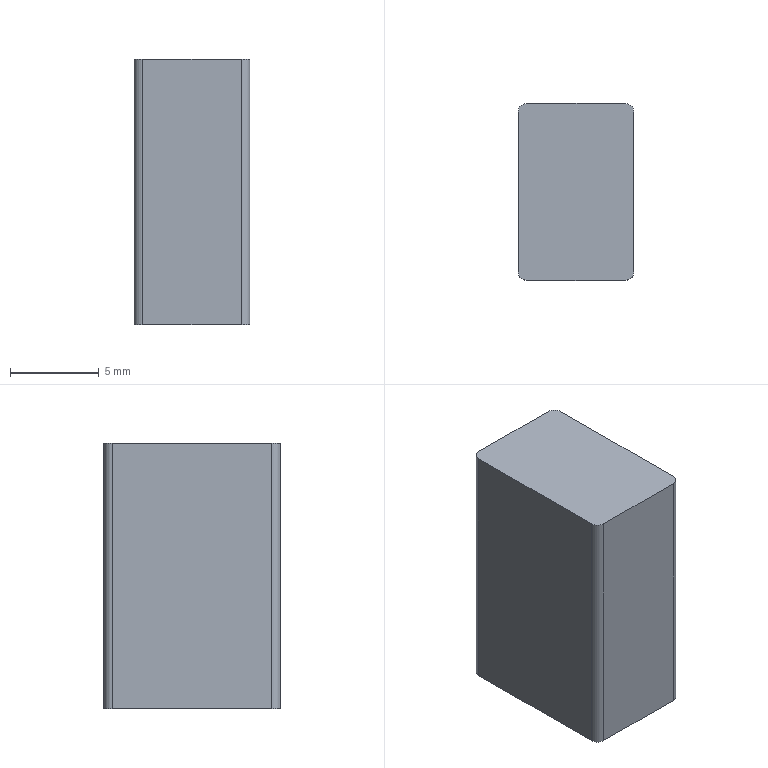Part | NX | features BREP 1 | 1 solid | 10 faces | box 6.547 x 9.991 x 15 mm | volume 978.032 mm3 | plane 6 | cylinder 4 | commonest cylinder face diameters 1 x4
STEP:
#1=CARTESIAN_POINT('',(-2.774,4.996,-25.6));
#2=VERTEX_POINT('',#1);
#3=CARTESIAN_POINT('',(-3.274,4.496,-25.6));
#4=VERTEX_POINT('',#3);
#5=CARTESIAN_POINT('',(-2.774,4.496,-25.6));
#6=DIRECTION('',(0.,0.,1.));
#7=DIRECTION('',(1.,0.,0.));
#8=AXIS2_PLACEMENT_3D('',#5,#6,#7);
#9=CIRCLE('',#8,0.5);
#10=EDGE_CURVE('',#2,#4,#9,.T.);
#11=ORIENTED_EDGE('',*,*,#10,.F.);
#12=CARTESIAN_POINT('',(-2.774,4.996,-40.6));
#13=VERTEX_POINT('',#12);
#14=CARTESIAN_POINT('',(-2.774,4.996,-40.6));
#15=DIRECTION('',(0.,0.,1.));
#16=VECTOR('',#15,1000.);
#17=LINE('',#14,#16);
#18=EDGE_CURVE('',#13,#2,#17,.T.);
#19=ORIENTED_EDGE('',*,*,#18,.F.);
#20=CARTESIAN_POINT('',(-3.274,4.496,-40.6));
#21=VERTEX_POINT('',#20);
#22=CARTESIAN_POINT('',(-2.774,4.496,-40.6));
#23=DIRECTION('',(0.,0.,1.));
#24=DIRECTION('',(1.,0.,0.));
#25=AXIS2_PLACEMENT_3D('',#22,#23,#24);
#26=CIRCLE('',#25,0.5);
#27=EDGE_CURVE('',#13,#21,#26,.T.);
#28=ORIENTED_EDGE('',*,*,#27,.T.);
#29=CARTESIAN_POINT('',(-3.274,4.496,-40.6));
#30=DIRECTION('',(0.,0.,1.));
#31=VECTOR('',#30,1000.);
#32=LINE('',#29,#31);
#33=EDGE_CURVE('',#21,#4,#32,.T.);
#34=ORIENTED_EDGE('',*,*,#33,.T.);
#35=EDGE_LOOP('',(#11,#19,#28,#34));
#36=FACE_BOUND('',#35,.T.);
#37=CARTESIAN_POINT('',(-2.774,4.496,-40.6));
#38=DIRECTION('',(0.,0.,1.));
#39=DIRECTION('',(-1.,0.,0.));
#40=AXIS2_PLACEMENT_3D('',#37,#38,#39);
#41=CYLINDRICAL_SURFACE('',#40,0.5);
#42=ADVANCED_FACE('',(#36),#41,.T.);
#43=CARTESIAN_POINT('',(-3.274,-4.496,-25.6));
#44=VERTEX_POINT('',#43);
#45=CARTESIAN_POINT('',(-3.274,-4.496,-25.6));
#46=DIRECTION('',(0.,1.,0.));
#47=VECTOR('',#46,1000.);
#48=LINE('',#45,#47);
#49=EDGE_CURVE('',#44,#4,#48,.T.);
#50=ORIENTED_EDGE('',*,*,#49,.T.);
#51=ORIENTED_EDGE('',*,*,#33,.F.);
#52=CARTESIAN_POINT('',(-3.274,-4.496,-40.6));
#53=VERTEX_POINT('',#52);
#54=CARTESIAN_POINT('',(-3.274,-4.496,-40.6));
#55=DIRECTION('',(0.,1.,0.));
#56=VECTOR('',#55,1000.);
#57=LINE('',#54,#56);
#58=EDGE_CURVE('',#53,#21,#57,.T.);
#59=ORIENTED_EDGE('',*,*,#58,.F.);
#60=CARTESIAN_POINT('',(-3.274,-4.496,-40.6));
#61=DIRECTION('',(0.,0.,1.));
#62=VECTOR('',#61,1000.);
#63=LINE('',#60,#62);
#64=EDGE_CURVE('',#53,#44,#63,.T.);
#65=ORIENTED_EDGE('',*,*,#64,.T.);
#66=EDGE_LOOP('',(#50,#51,#59,#65));
#67=FACE_BOUND('',#66,.T.);
#68=CARTESIAN_POINT('',(-3.274,-4.496,-40.6));
#69=DIRECTION('',(1.,0.,0.));
#70=DIRECTION('',(0.,-1.,0.));
#71=AXIS2_PLACEMENT_3D('',#68,#69,#70);
#72=PLANE('',#71);
#73=ADVANCED_FACE('',(#67),#72,.F.);
#74=CARTESIAN_POINT('',(-2.774,-4.996,-25.6));
#75=VERTEX_POINT('',#74);
#76=CARTESIAN_POINT('',(-2.774,-4.496,-25.6));
#77=DIRECTION('',(0.,0.,1.));
#78=DIRECTION('',(1.,0.,0.));
#79=AXIS2_PLACEMENT_3D('',#76,#77,#78);
#80=CIRCLE('',#79,0.5);
#81=EDGE_CURVE('',#44,#75,#80,.T.);
#82=ORIENTED_EDGE('',*,*,#81,.F.);
#83=ORIENTED_EDGE('',*,*,#64,.F.);
#84=CARTESIAN_POINT('',(-2.774,-4.996,-40.6));
#85=VERTEX_POINT('',#84);
#86=CARTESIAN_POINT('',(-2.774,-4.496,-40.6));
#87=DIRECTION('',(0.,0.,1.));
#88=DIRECTION('',(1.,0.,0.));
#89=AXIS2_PLACEMENT_3D('',#86,#87,#88);
#90=CIRCLE('',#89,0.5);
#91=EDGE_CURVE('',#53,#85,#90,.T.);
#92=ORIENTED_EDGE('',*,*,#91,.T.);
#93=CARTESIAN_POINT('',(-2.774,-4.996,-40.6));
#94=DIRECTION('',(0.,0.,1.));
#95=VECTOR('',#94,1000.);
#96=LINE('',#93,#95);
#97=EDGE_CURVE('',#85,#75,#96,.T.);
#98=ORIENTED_EDGE('',*,*,#97,.T.);
#99=EDGE_LOOP('',(#82,#83,#92,#98));
#100=FACE_BOUND('',#99,.T.);
#101=CARTESIAN_POINT('',(-2.774,-4.496,-40.6));
#102=DIRECTION('',(0.,0.,1.));
#103=DIRECTION('',(-1.,0.,0.));
#104=AXIS2_PLACEMENT_3D('',#101,#102,#103);
#105=CYLINDRICAL_SURFACE('',#104,0.5);
#106=ADVANCED_FACE('',(#100),#105,.T.);
#107=CARTESIAN_POINT('',(2.774,-4.996,-25.6));
#108=VERTEX_POINT('',#107);
#109=CARTESIAN_POINT('',(2.774,-4.996,-25.6));
#110=DIRECTION('',(-1.,0.,0.));
#111=VECTOR('',#110,1000.);
#112=LINE('',#109,#111);
#113=EDGE_CURVE('',#108,#75,#112,.T.);
#114=ORIENTED_EDGE('',*,*,#113,.T.);
#115=ORIENTED_EDGE('',*,*,#97,.F.);
#116=CARTESIAN_POINT('',(2.774,-4.996,-40.6));
#117=VERTEX_POINT('',#116);
#118=CARTESIAN_POINT('',(2.774,-4.996,-40.6));
#119=DIRECTION('',(-1.,0.,0.));
#120=VECTOR('',#119,1000.);
#121=LINE('',#118,#120);
#122=EDGE_CURVE('',#117,#85,#121,.T.);
#123=ORIENTED_EDGE('',*,*,#122,.F.);
#124=CARTESIAN_POINT('',(2.774,-4.996,-40.6));
#125=DIRECTION('',(0.,0.,1.));
#126=VECTOR('',#125,1000.);
#127=LINE('',#124,#126);
#128=EDGE_CURVE('',#117,#108,#127,.T.);
#129=ORIENTED_EDGE('',*,*,#128,.T.);
#130=EDGE_LOOP('',(#114,#115,#123,#129));
#131=FACE_BOUND('',#130,.T.);
#132=CARTESIAN_POINT('',(2.774,-4.996,-40.6));
#133=DIRECTION('',(0.,1.,0.));
#134=DIRECTION('',(0.,0.,-1.));
#135=AXIS2_PLACEMENT_3D('',#132,#133,#134);
#136=PLANE('',#135);
#137=ADVANCED_FACE('',(#131),#136,.F.);
#138=CARTESIAN_POINT('',(3.274,-4.496,-25.6));
#139=VERTEX_POINT('',#138);
#140=CARTESIAN_POINT('',(2.774,-4.496,-25.6));
#141=DIRECTION('',(0.,0.,1.));
#142=DIRECTION('',(1.,0.,0.));
#143=AXIS2_PLACEMENT_3D('',#140,#141,#142);
#144=CIRCLE('',#143,0.5);
#145=EDGE_CURVE('',#108,#139,#144,.T.);
#146=ORIENTED_EDGE('',*,*,#145,.F.);
#147=ORIENTED_EDGE('',*,*,#128,.F.);
#148=CARTESIAN_POINT('',(3.274,-4.496,-40.6));
#149=VERTEX_POINT('',#148);
#150=CARTESIAN_POINT('',(2.774,-4.496,-40.6));
#151=DIRECTION('',(0.,0.,1.));
#152=DIRECTION('',(1.,0.,0.));
#153=AXIS2_PLACEMENT_3D('',#150,#151,#152);
#154=CIRCLE('',#153,0.5);
#155=EDGE_CURVE('',#117,#149,#154,.T.);
#156=ORIENTED_EDGE('',*,*,#155,.T.);
#157=CARTESIAN_POINT('',(3.274,-4.496,-40.6));
#158=DIRECTION('',(0.,0.,1.));
#159=VECTOR('',#158,1000.);
#160=LINE('',#157,#159);
#161=EDGE_CURVE('',#149,#139,#160,.T.);
#162=ORIENTED_EDGE('',*,*,#161,.T.);
#163=EDGE_LOOP('',(#146,#147,#156,#162));
#164=FACE_BOUND('',#163,.T.);
#165=CARTESIAN_POINT('',(2.774,-4.496,-40.6));
#166=DIRECTION('',(0.,0.,1.));
#167=DIRECTION('',(-1.,0.,0.));
#168=AXIS2_PLACEMENT_3D('',#165,#166,#167);
#169=CYLINDRICAL_SURFACE('',#168,0.5);
#170=ADVANCED_FACE('',(#164),#169,.T.);
#171=CARTESIAN_POINT('',(3.274,4.496,-25.6));
#172=VERTEX_POINT('',#171);
#173=CARTESIAN_POINT('',(3.274,4.496,-25.6));
#174=DIRECTION('',(0.,-1.,0.));
#175=VECTOR('',#174,1000.);
#176=LINE('',#173,#175);
#177=EDGE_CURVE('',#172,#139,#176,.T.);
#178=ORIENTED_EDGE('',*,*,#177,.T.);
#179=ORIENTED_EDGE('',*,*,#161,.F.);
#180=CARTESIAN_POINT('',(3.274,4.496,-40.6));
#181=VERTEX_POINT('',#180);
#182=CARTESIAN_POINT('',(3.274,4.496,-40.6));
#183=DIRECTION('',(0.,-1.,0.));
#184=VECTOR('',#183,1000.);
#185=LINE('',#182,#184);
#186=EDGE_CURVE('',#181,#149,#185,.T.);
#187=ORIENTED_EDGE('',*,*,#186,.F.);
#188=CARTESIAN_POINT('',(3.274,4.496,-40.6));
#189=DIRECTION('',(0.,0.,1.));
#190=VECTOR('',#189,1000.);
#191=LINE('',#188,#190);
#192=EDGE_CURVE('',#181,#172,#191,.T.);
#193=ORIENTED_EDGE('',*,*,#192,.T.);
#194=EDGE_LOOP('',(#178,#179,#187,#193));
#195=FACE_BOUND('',#194,.T.);
#196=CARTESIAN_POINT('',(3.274,4.496,-40.6));
#197=DIRECTION('',(-1.,0.,0.));
#198=DIRECTION('',(0.,1.,0.));
#199=AXIS2_PLACEMENT_3D('',#196,#197,#198);
#200=PLANE('',#199);
#201=ADVANCED_FACE('',(#195),#200,.F.);
#202=CARTESIAN_POINT('',(2.774,4.996,-25.6));
#203=VERTEX_POINT('',#202);
#204=CARTESIAN_POINT('',(2.774,4.496,-25.6));
#205=DIRECTION('',(0.,0.,1.));
#206=DIRECTION('',(1.,0.,0.));
#207=AXIS2_PLACEMENT_3D('',#204,#205,#206);
#208=CIRCLE('',#207,0.5);
#209=EDGE_CURVE('',#172,#203,#208,.T.);
#210=ORIENTED_EDGE('',*,*,#209,.F.);
#211=ORIENTED_EDGE('',*,*,#192,.F.);
#212=CARTESIAN_POINT('',(2.774,4.996,-40.6));
#213=VERTEX_POINT('',#212);
#214=CARTESIAN_POINT('',(2.774,4.496,-40.6));
#215=DIRECTION('',(0.,0.,1.));
#216=DIRECTION('',(1.,0.,0.));
#217=AXIS2_PLACEMENT_3D('',#214,#215,#216);
#218=CIRCLE('',#217,0.5);
#219=EDGE_CURVE('',#181,#213,#218,.T.);
#220=ORIENTED_EDGE('',*,*,#219,.T.);
#221=CARTESIAN_POINT('',(2.774,4.996,-40.6));
#222=DIRECTION('',(0.,0.,1.));
#223=VECTOR('',#222,1000.);
#224=LINE('',#221,#223);
#225=EDGE_CURVE('',#213,#203,#224,.T.);
#226=ORIENTED_EDGE('',*,*,#225,.T.);
#227=EDGE_LOOP('',(#210,#211,#220,#226));
#228=FACE_BOUND('',#227,.T.);
#229=CARTESIAN_POINT('',(2.774,4.496,-40.6));
#230=DIRECTION('',(0.,0.,1.));
#231=DIRECTION('',(-1.,0.,0.));
#232=AXIS2_PLACEMENT_3D('',#229,#230,#231);
#233=CYLINDRICAL_SURFACE('',#232,0.5);
#234=ADVANCED_FACE('',(#228),#233,.T.);
#235=CARTESIAN_POINT('',(-2.774,4.996,-25.6));
#236=DIRECTION('',(1.,0.,0.));
#237=VECTOR('',#236,1000.);
#238=LINE('',#235,#237);
#239=EDGE_CURVE('',#2,#203,#238,.T.);
#240=ORIENTED_EDGE('',*,*,#239,.T.);
#241=ORIENTED_EDGE('',*,*,#225,.F.);
#242=CARTESIAN_POINT('',(-2.774,4.996,-40.6));
#243=DIRECTION('',(1.,0.,0.));
#244=VECTOR('',#243,1000.);
#245=LINE('',#242,#244);
#246=EDGE_CURVE('',#13,#213,#245,.T.);
#247=ORIENTED_EDGE('',*,*,#246,.F.);
#248=ORIENTED_EDGE('',*,*,#18,.T.);
#249=EDGE_LOOP('',(#240,#241,#247,#248));
#250=FACE_BOUND('',#249,.T.);
#251=CARTESIAN_POINT('',(-2.774,4.996,-40.6));
#252=DIRECTION('',(0.,-1.,0.));
#253=DIRECTION('',(0.,0.,1.));
#254=AXIS2_PLACEMENT_3D('',#251,#252,#253);
#255=PLANE('',#254);
#256=ADVANCED_FACE('',(#250),#255,.F.);
#257=ORIENTED_EDGE('',*,*,#27,.F.);
#258=ORIENTED_EDGE('',*,*,#246,.T.);
#259=ORIENTED_EDGE('',*,*,#219,.F.);
#260=ORIENTED_EDGE('',*,*,#186,.T.);
#261=ORIENTED_EDGE('',*,*,#155,.F.);
#262=ORIENTED_EDGE('',*,*,#122,.T.);
#263=ORIENTED_EDGE('',*,*,#91,.F.);
#264=ORIENTED_EDGE('',*,*,#58,.T.);
#265=EDGE_LOOP('',(#257,#258,#259,#260,#261,#262,#263,#264));
#266=FACE_BOUND('',#265,.T.);
#267=CARTESIAN_POINT('',(-2.774,4.496,-40.6));
#268=DIRECTION('',(0.,0.,1.));
#269=DIRECTION('',(-1.,0.,0.));
#270=AXIS2_PLACEMENT_3D('',#267,#268,#269);
#271=PLANE('',#270);
#272=ADVANCED_FACE('',(#266),#271,.F.);
#273=ORIENTED_EDGE('',*,*,#10,.T.);
#274=ORIENTED_EDGE('',*,*,#49,.F.);
#275=ORIENTED_EDGE('',*,*,#81,.T.);
#276=ORIENTED_EDGE('',*,*,#113,.F.);
#277=ORIENTED_EDGE('',*,*,#145,.T.);
#278=ORIENTED_EDGE('',*,*,#177,.F.);
#279=ORIENTED_EDGE('',*,*,#209,.T.);
#280=ORIENTED_EDGE('',*,*,#239,.F.);
#281=EDGE_LOOP('',(#273,#274,#275,#276,#277,#278,#279,#280));
#282=FACE_BOUND('',#281,.T.);
#283=CARTESIAN_POINT('',(-2.774,4.496,-25.6));
#284=DIRECTION('',(0.,0.,1.));
#285=DIRECTION('',(-1.,0.,0.));
#286=AXIS2_PLACEMENT_3D('',#283,#284,#285);
#287=PLANE('',#286);
#288=ADVANCED_FACE('',(#282),#287,.T.);
#289=CLOSED_SHELL('',(#42,#73,#106,#137,#170,#201,#234,#256,#272,#288));
#290=MANIFOLD_SOLID_BREP('',#289);
#291=(LENGTH_UNIT()NAMED_UNIT(*)SI_UNIT(.MILLI.,.METRE.));
#292=UNCERTAINTY_MEASURE_WITH_UNIT(LENGTH_MEASURE(0.00001),#291,'','');
#293=(NAMED_UNIT(*)PLANE_ANGLE_UNIT()SI_UNIT($,.RADIAN.));
#294=(NAMED_UNIT(*)SI_UNIT($,.STERADIAN.)SOLID_ANGLE_UNIT());
#295=(GEOMETRIC_REPRESENTATION_CONTEXT(3)GLOBAL_UNCERTAINTY_ASSIGNED_CONTEXT((#292))GLOBAL_UNIT_ASSIGNED_CONTEXT((#291,#293,#294))REPRESENTATION_CONTEXT('',''));
#296=ADVANCED_BREP_SHAPE_REPRESENTATION('',(#290),#295);